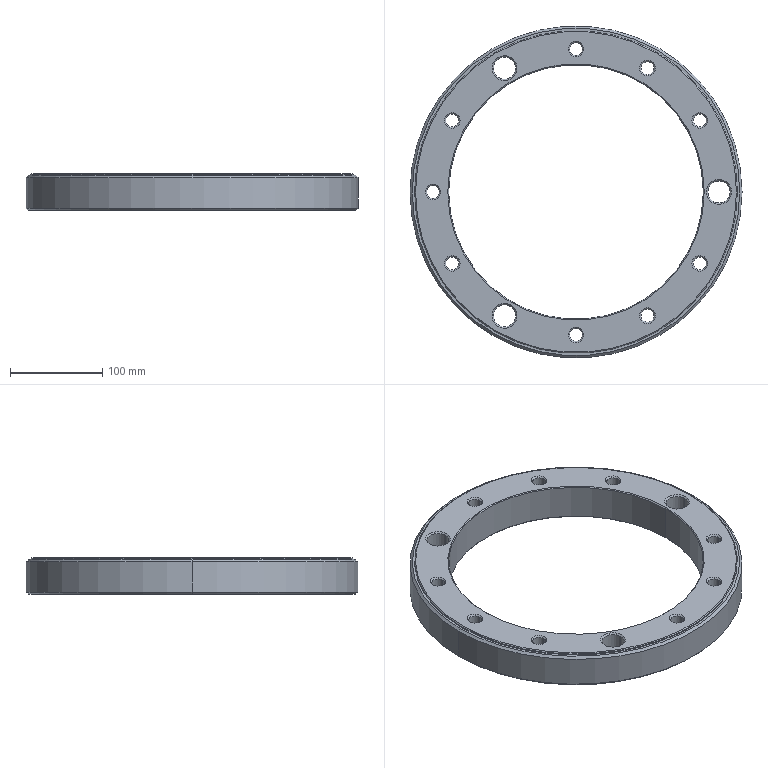Part | NX | features BREP 1 | 1 solid | 91 faces | box 360 x 360 x 40 mm | volume 1547569 mm3 | cone 58 | cylinder 30 | plane 3 | commonest cylinder face diameters 14 x18 24 x6 276 x2 350 x2 360 x2